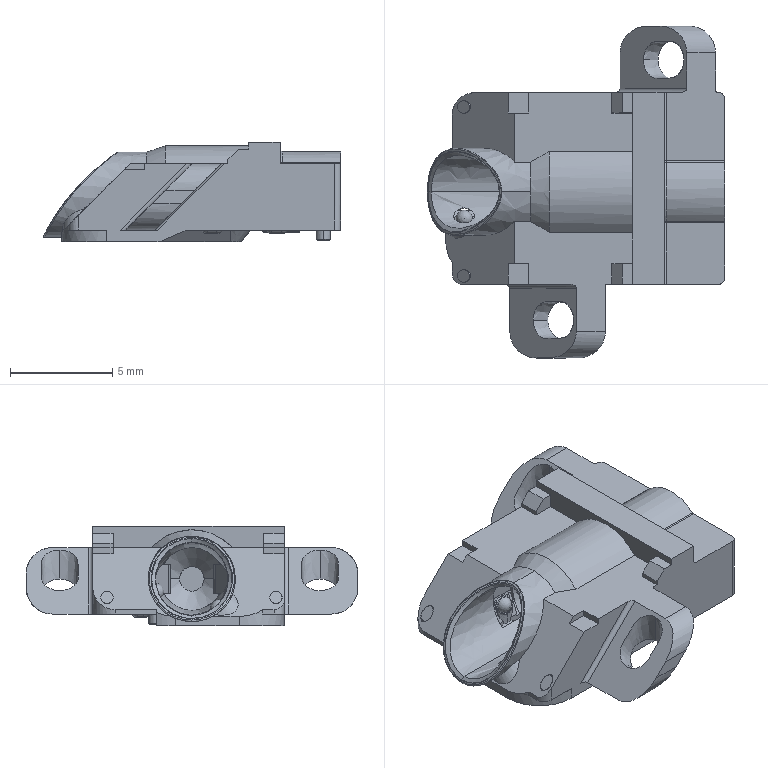Part | NX | 5 solids | 1004 faces | box 14.51 x 16.208 x 4.858 mm | volume 286.621 mm3 | plane 542 | cylinder 298 | torus 99 | spline 27 | sphere 20 | cone 18 | commonest cylinder face diameters 0.2 x81 0.4 x26 1 x20 0.6 x19 0.3 x18 0.7 x18